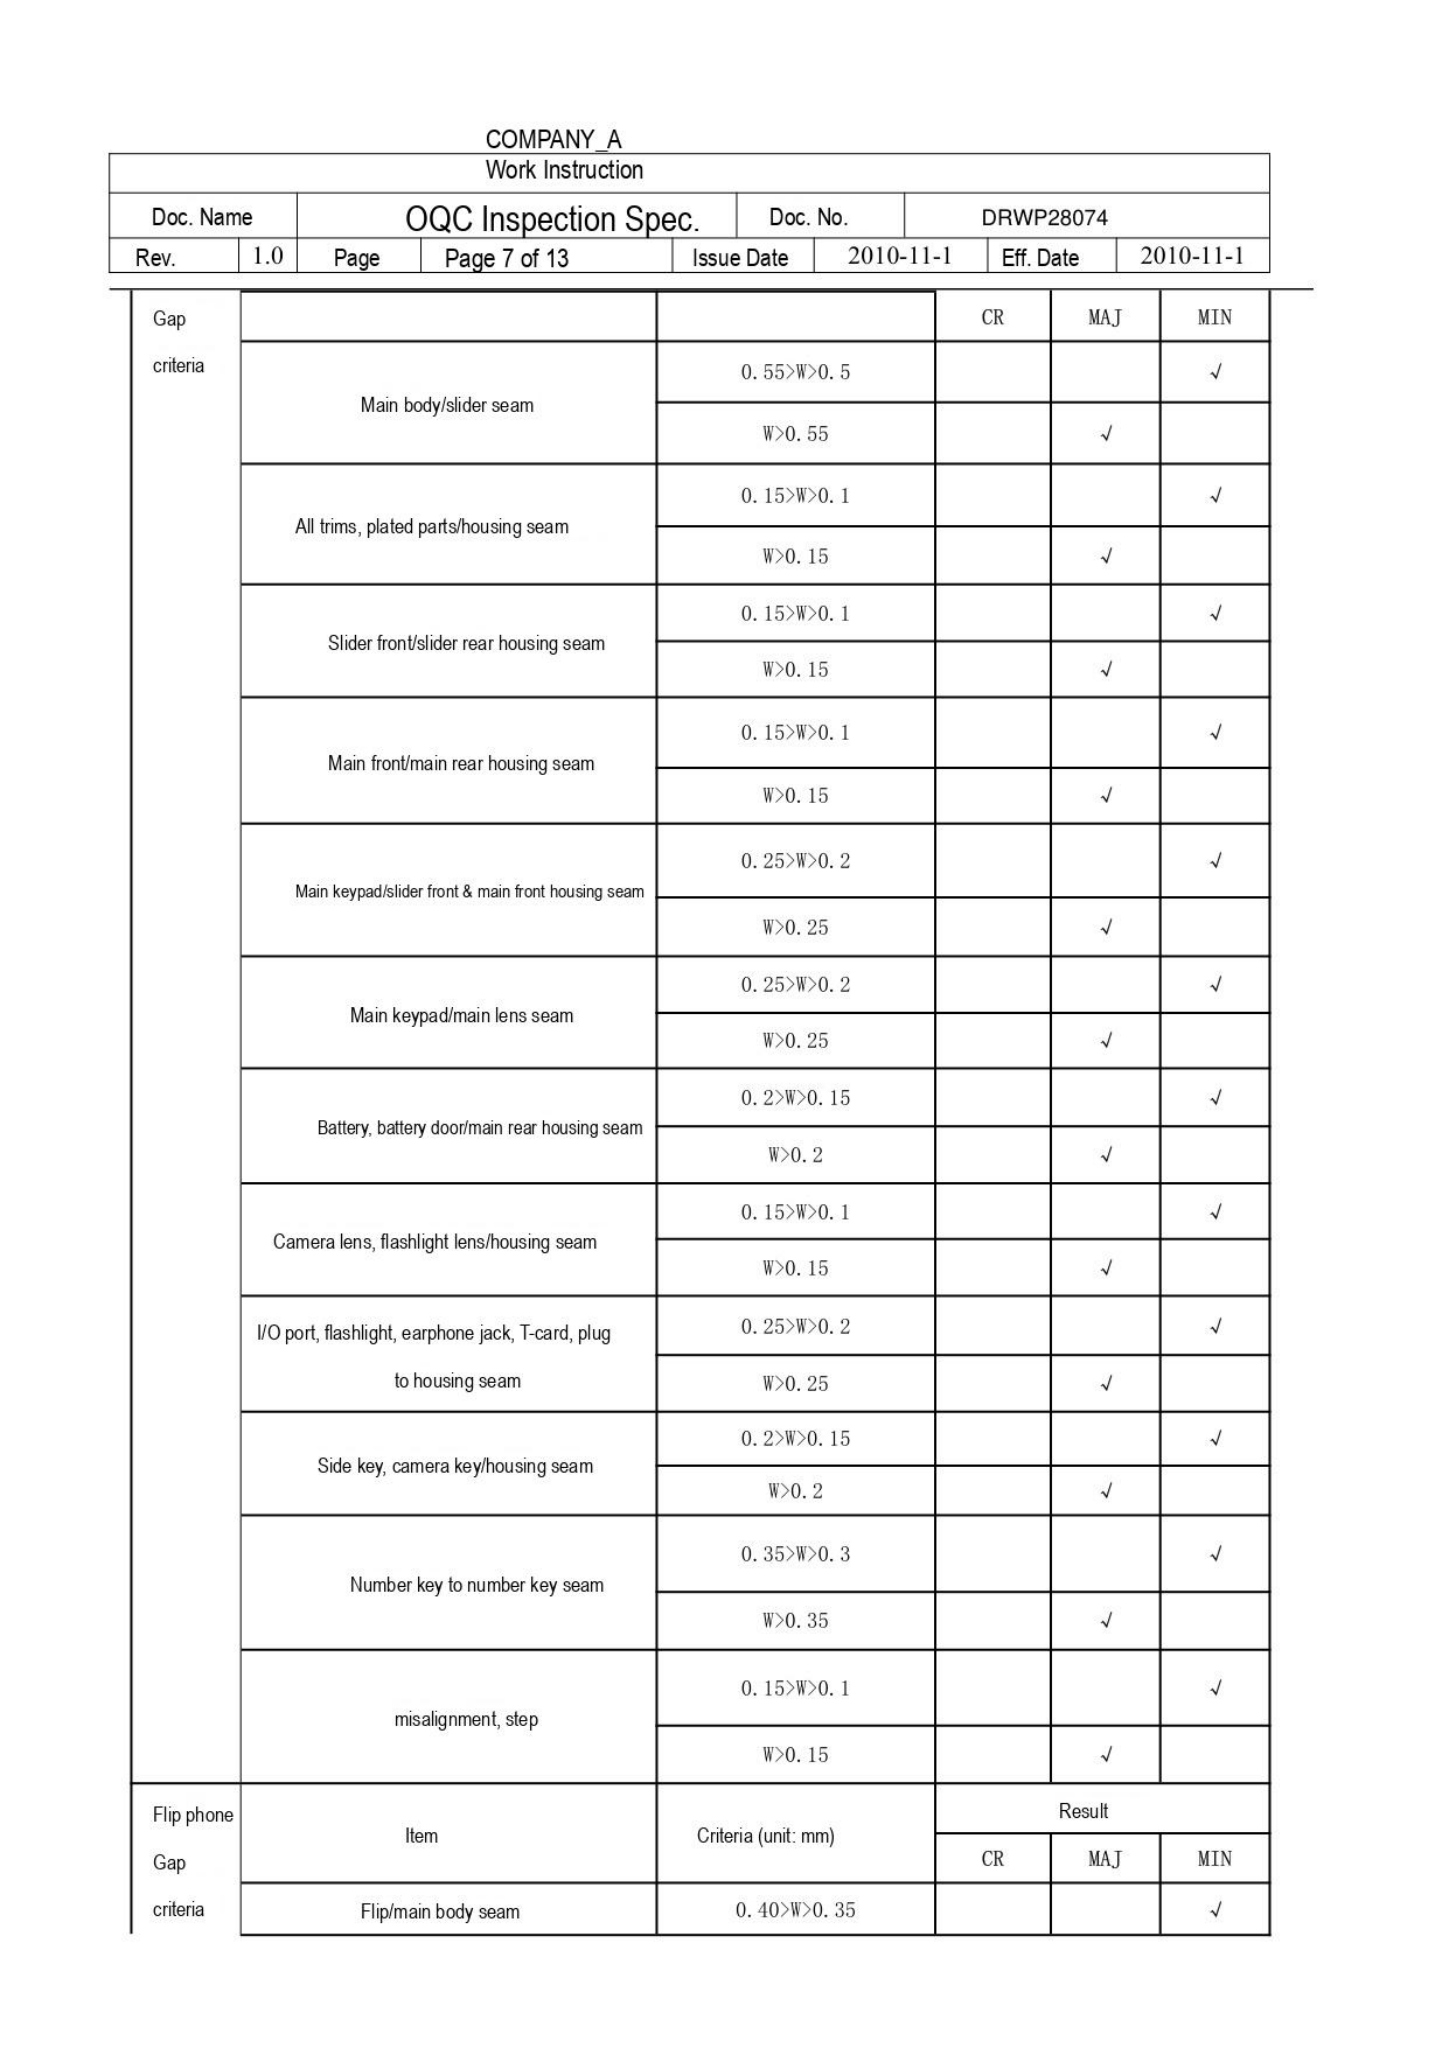COMPANY_A

| Work Instruction | | | | | | | |
|---|---|---|---|---|---|---|---|
| Doc. Name | OQC Inspection Spec. | | | Doc. No. | DRWP28074 | | |
| Rev. | 1.0 | Page | Page 7 of 13 | Issue Date | 2010-11-1 | Eff. Date | 2010-11-1 |

| Gap criteria | | | CR | MAJ | MIN |
|---|---|---|---|---|---|
| | Main body/slider seam | 0. 55>W>0. 5 | | | √ |
| | | W>0. 55 | | √ | |
| | All trims, plated parts/housing seam | 0. 15>W>0. 1 | | | √ |
| | | W>0. 15 | | √ | |
| | Slider front/slider rear housing seam | 0. 15>W>0. 1 | | | √ |
| | | W>0. 15 | | √ | |
| | Main front/main rear housing seam | 0. 15>W>0. 1 | | | √ |
| | | W>0. 15 | | √ | |
| | Main keypad/slider front & main front housing seam | 0. 25>W>0. 2 | | | √ |
| | | W>0. 25 | | √ | |
| | Main keypad/main lens seam | 0. 25>W>0. 2 | | | √ |
| | | W>0. 25 | | √ | |
| | Battery, battery door/main rear housing seam | 0. 2>W>0. 15 | | | √ |
| | | W>0. 2 | | √ | |
| | Camera lens, flashlight lens/housing seam | 0. 15>W>0. 1 | | | √ |
| | | W>0. 15 | | √ | |
| | I/O port, flashlight, earphone jack, T-card, plug to housing seam | 0. 25>W>0. 2 | | | √ |
| | | W>0. 25 | | √ | |
| | Side key, camera key/housing seam | 0. 2>W>0. 15 | | | √ |
| | | W>0. 2 | | √ | |
| | Number key to number key seam | 0. 35>W>0. 3 | | | √ |
| | | W>0. 35 | | √ | |
| | misalignment, step | 0. 15>W>0. 1 | | | √ |
| | | W>0. 15 | | √ | |

| Flip phone Gap criteria | Item | Criteria (unit: mm) | Result | | |
|---|---|---|---|---|---|
| | | | CR | MAJ | MIN |
| | Flip/main body seam | 0. 40>W>0. 35 | | | √ |
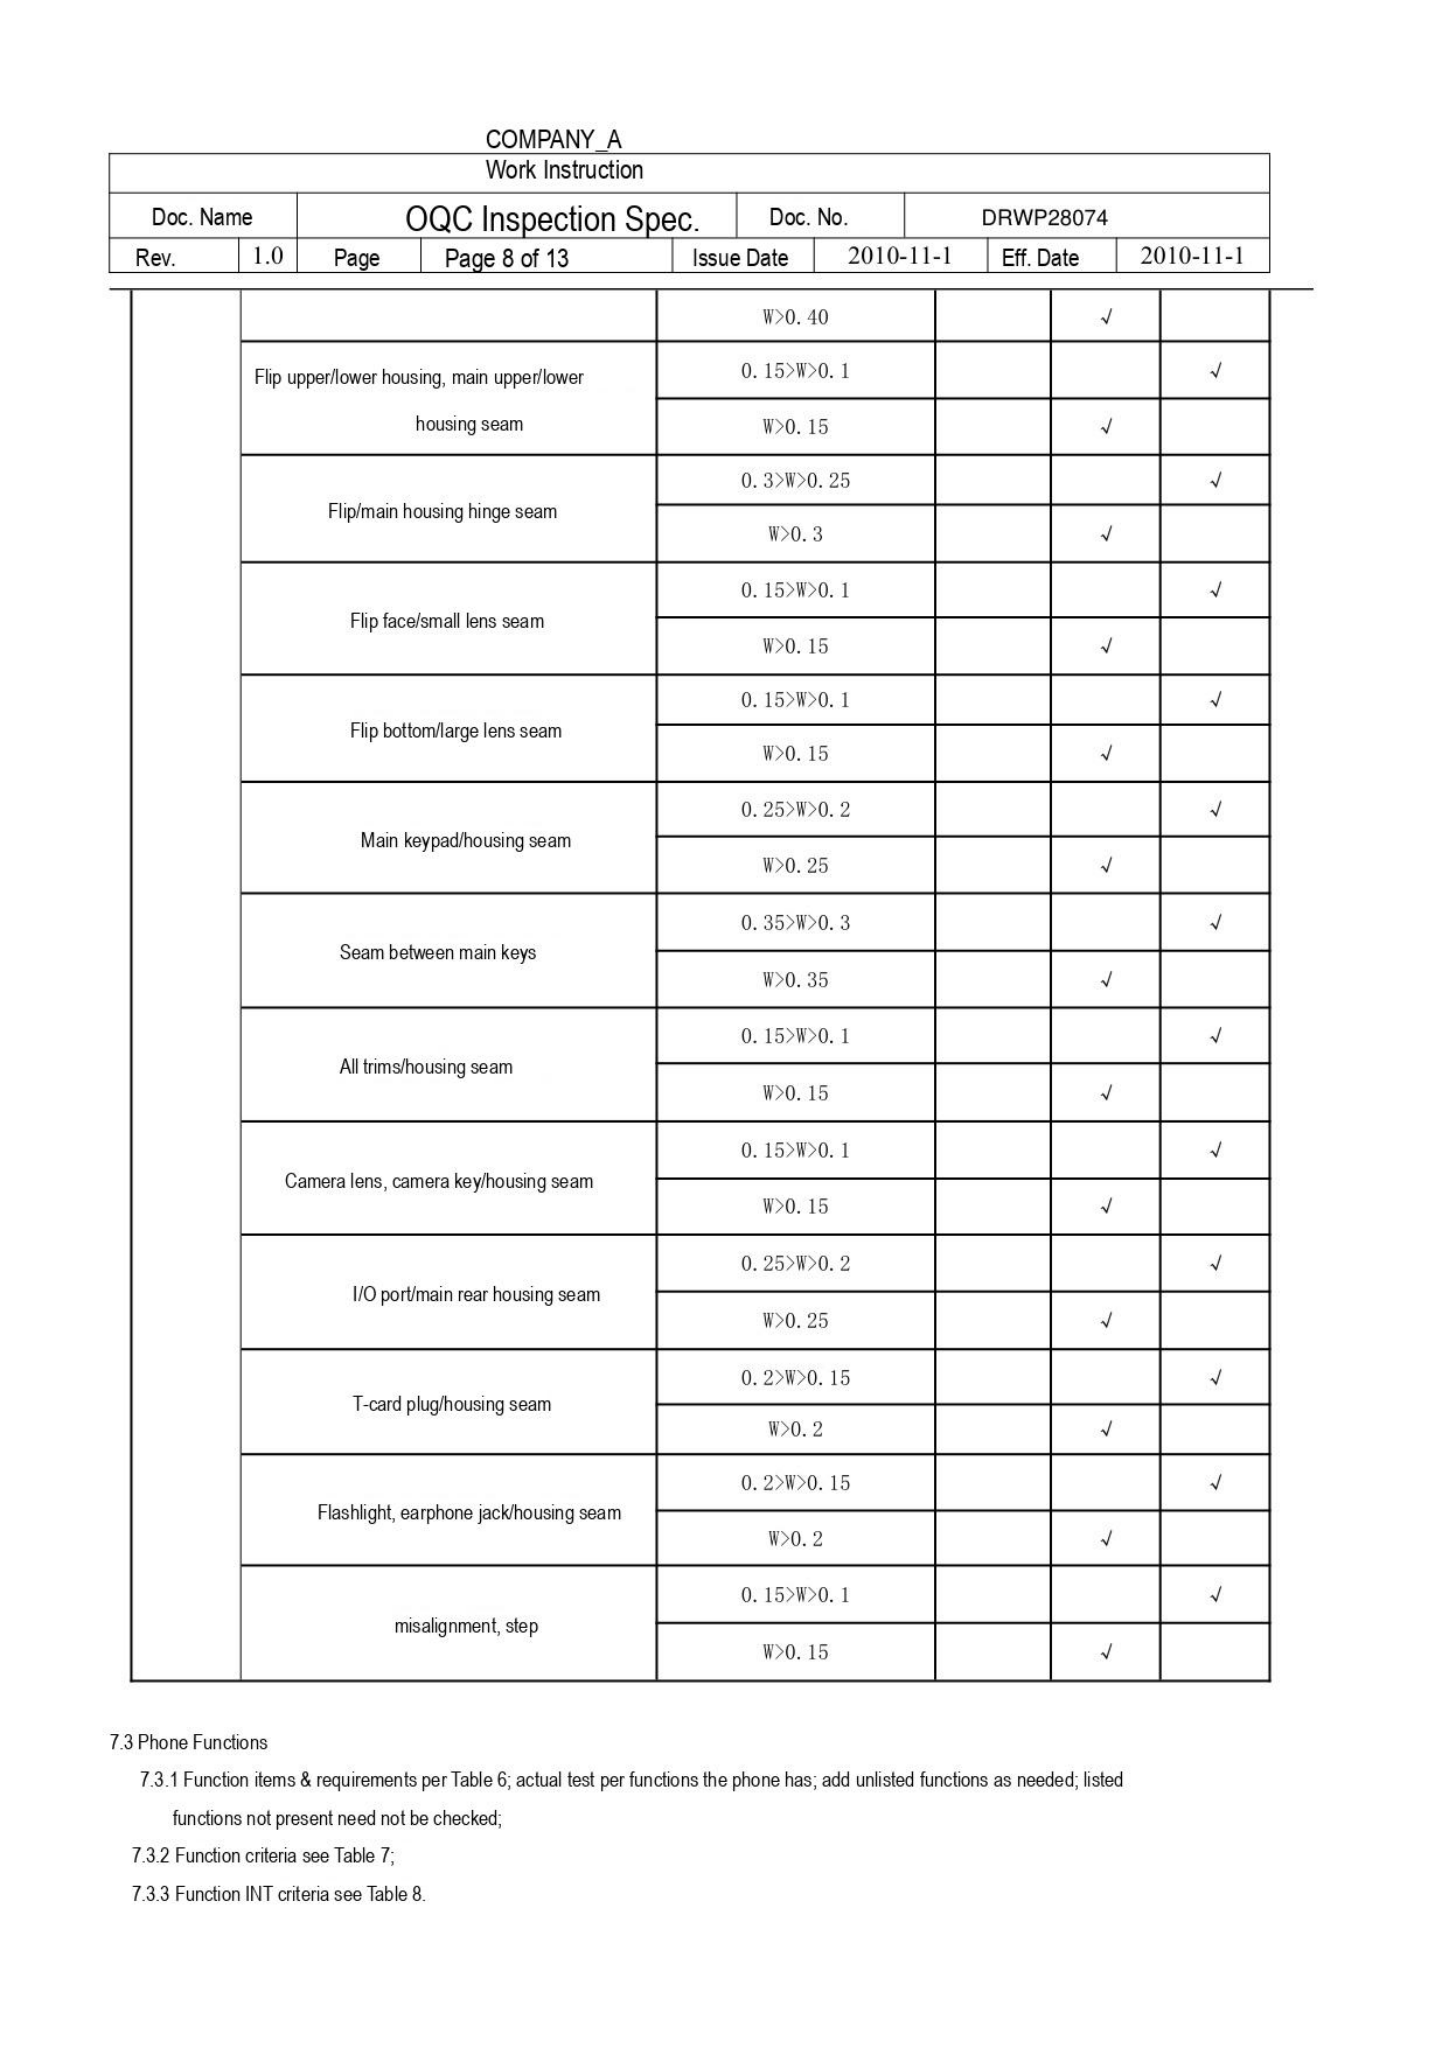COMPANY_A

| Work Instruction | | | | | | | |
|---|---|---|---|---|---|---|---|
| Doc. Name | | OQC Inspection Spec. | | Doc. No. | | DRWP28074 | |
| Rev. | 1.0 | Page | Page 8 of 13 | Issue Date | 2010-11-1 | Eff. Date | 2010-11-1 |

| | | | | | |
|---|---|---|---|---|---|
| | | W>0.40 | | √ | |
| | Flip upper/lower housing, main upper/lower housing seam | 0.15>W>0.1 | | | √ |
| | | W>0.15 | | √ | |
| | Flip/main housing hinge seam | 0.3>W>0.25 | | | √ |
| | | W>0.3 | | √ | |
| | Flip face/small lens seam | 0.15>W>0.1 | | | √ |
| | | W>0.15 | | √ | |
| | Flip bottom/large lens seam | 0.15>W>0.1 | | | √ |
| | | W>0.15 | | √ | |
| | Main keypad/housing seam | 0.25>W>0.2 | | | √ |
| | | W>0.25 | | √ | |
| | Seam between main keys | 0.35>W>0.3 | | | √ |
| | | W>0.35 | | √ | |
| | All trims/housing seam | 0.15>W>0.1 | | | √ |
| | | W>0.15 | | √ | |
| | Camera lens, camera key/housing seam | 0.15>W>0.1 | | | √ |
| | | W>0.15 | | √ | |
| | I/O port/main rear housing seam | 0.25>W>0.2 | | | √ |
| | | W>0.25 | | √ | |
| | T-card plug/housing seam | 0.2>W>0.15 | | | √ |
| | | W>0.2 | | √ | |
| | Flashlight, earphone jack/housing seam | 0.2>W>0.15 | | | √ |
| | | W>0.2 | | √ | |
| | misalignment, step | 0.15>W>0.1 | | | √ |
| | | W>0.15 | | √ | |

7.3 Phone Functions

7.3.1 Function items & requirements per Table 6; actual test per functions the phone has; add unlisted functions as needed; listed functions not present need not be checked;

7.3.2 Function criteria see Table 7;

7.3.3 Function INT criteria see Table 8.
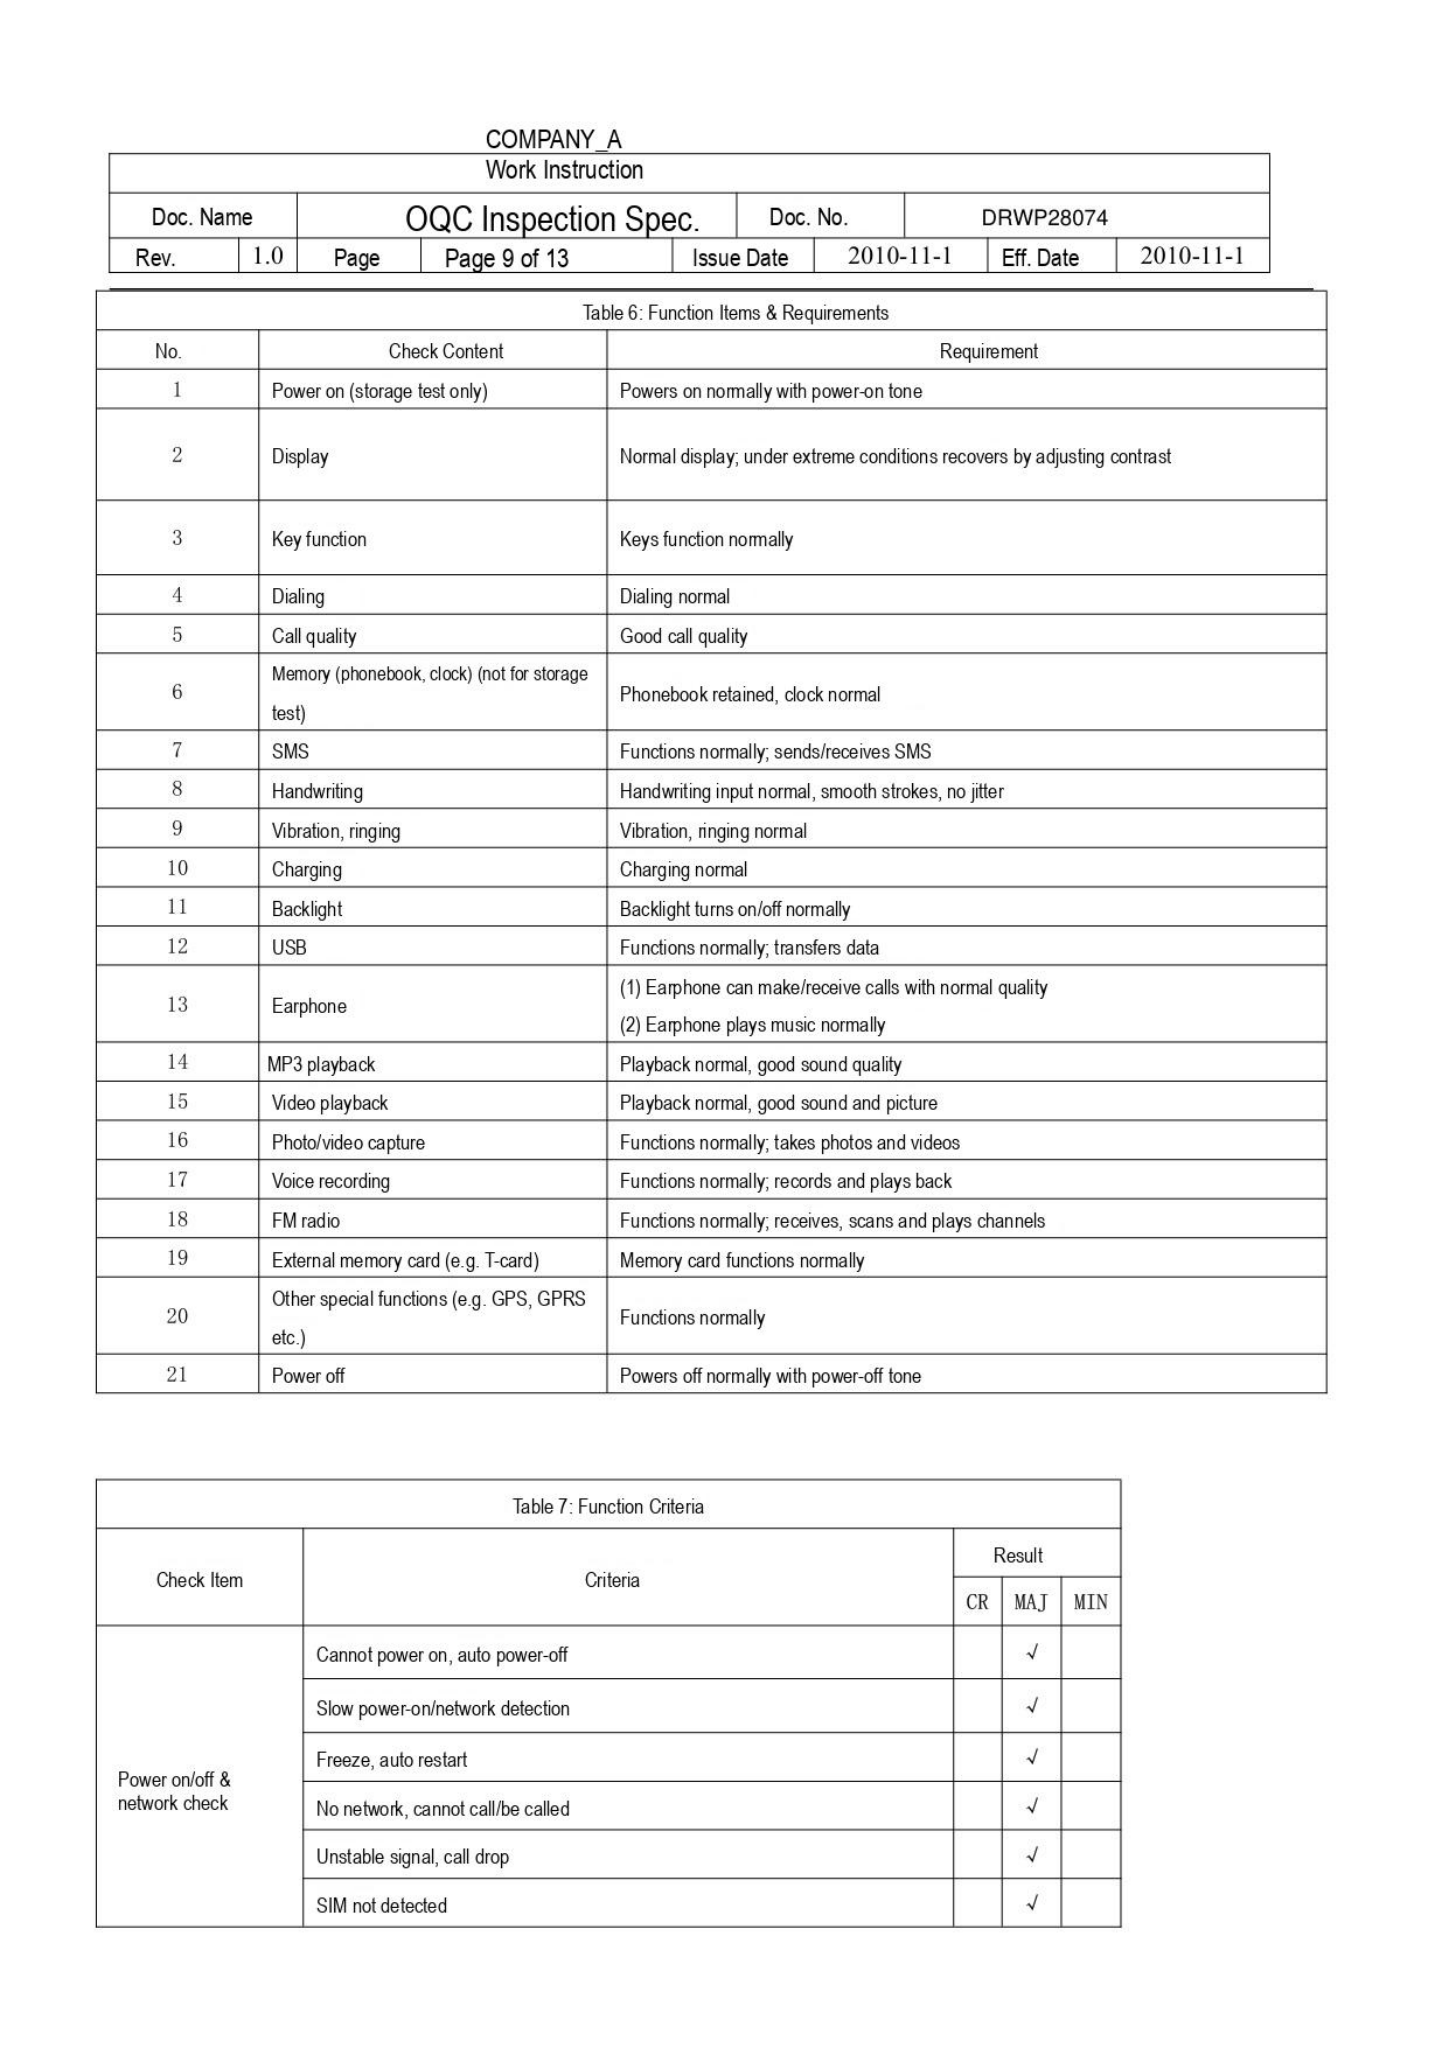COMPANY_A

| Work Instruction | | | | | | | |
|---|---|---|---|---|---|---|---|
| Doc. Name | | OQC Inspection Spec. | | Doc. No. | | DRWP28074 | |
| Rev. | 1.0 | Page | Page 9 of 13 | Issue Date | 2010-11-1 | Eff. Date | 2010-11-1 |

Table 6: Function Items & Requirements

| No. | Check Content | Requirement |
|---|---|---|
| 1 | Power on (storage test only) | Powers on normally with power-on tone |
| 2 | Display | Normal display; under extreme conditions recovers by adjusting contrast |
| 3 | Key function | Keys function normally |
| 4 | Dialing | Dialing normal |
| 5 | Call quality | Good call quality |
| 6 | Memory (phonebook, clock) (not for storage test) | Phonebook retained, clock normal |
| 7 | SMS | Functions normally; sends/receives SMS |
| 8 | Handwriting | Handwriting input normal, smooth strokes, no jitter |
| 9 | Vibration, ringing | Vibration, ringing normal |
| 10 | Charging | Charging normal |
| 11 | Backlight | Backlight turns on/off normally |
| 12 | USB | Functions normally; transfers data |
| 13 | Earphone | (1) Earphone can make/receive calls with normal quality<br>(2) Earphone plays music normally |
| 14 | MP3 playback | Playback normal, good sound quality |
| 15 | Video playback | Playback normal, good sound and picture |
| 16 | Photo/video capture | Functions normally; takes photos and videos |
| 17 | Voice recording | Functions normally; records and plays back |
| 18 | FM radio | Functions normally; receives, scans and plays channels |
| 19 | External memory card (e.g. T-card) | Memory card functions normally |
| 20 | Other special functions (e.g. GPS, GPRS etc.) | Functions normally |
| 21 | Power off | Powers off normally with power-off tone |

Table 7: Function Criteria

| Check Item | Criteria | Result: CR | Result: MAJ | Result: MIN |
|---|---|---|---|---|
| Power on/off & network check | Cannot power on, auto power-off | | √ | |
| | Slow power-on/network detection | | √ | |
| | Freeze, auto restart | | √ | |
| | No network, cannot call/be called | | √ | |
| | Unstable signal, call drop | | √ | |
| | SIM not detected | | √ | |
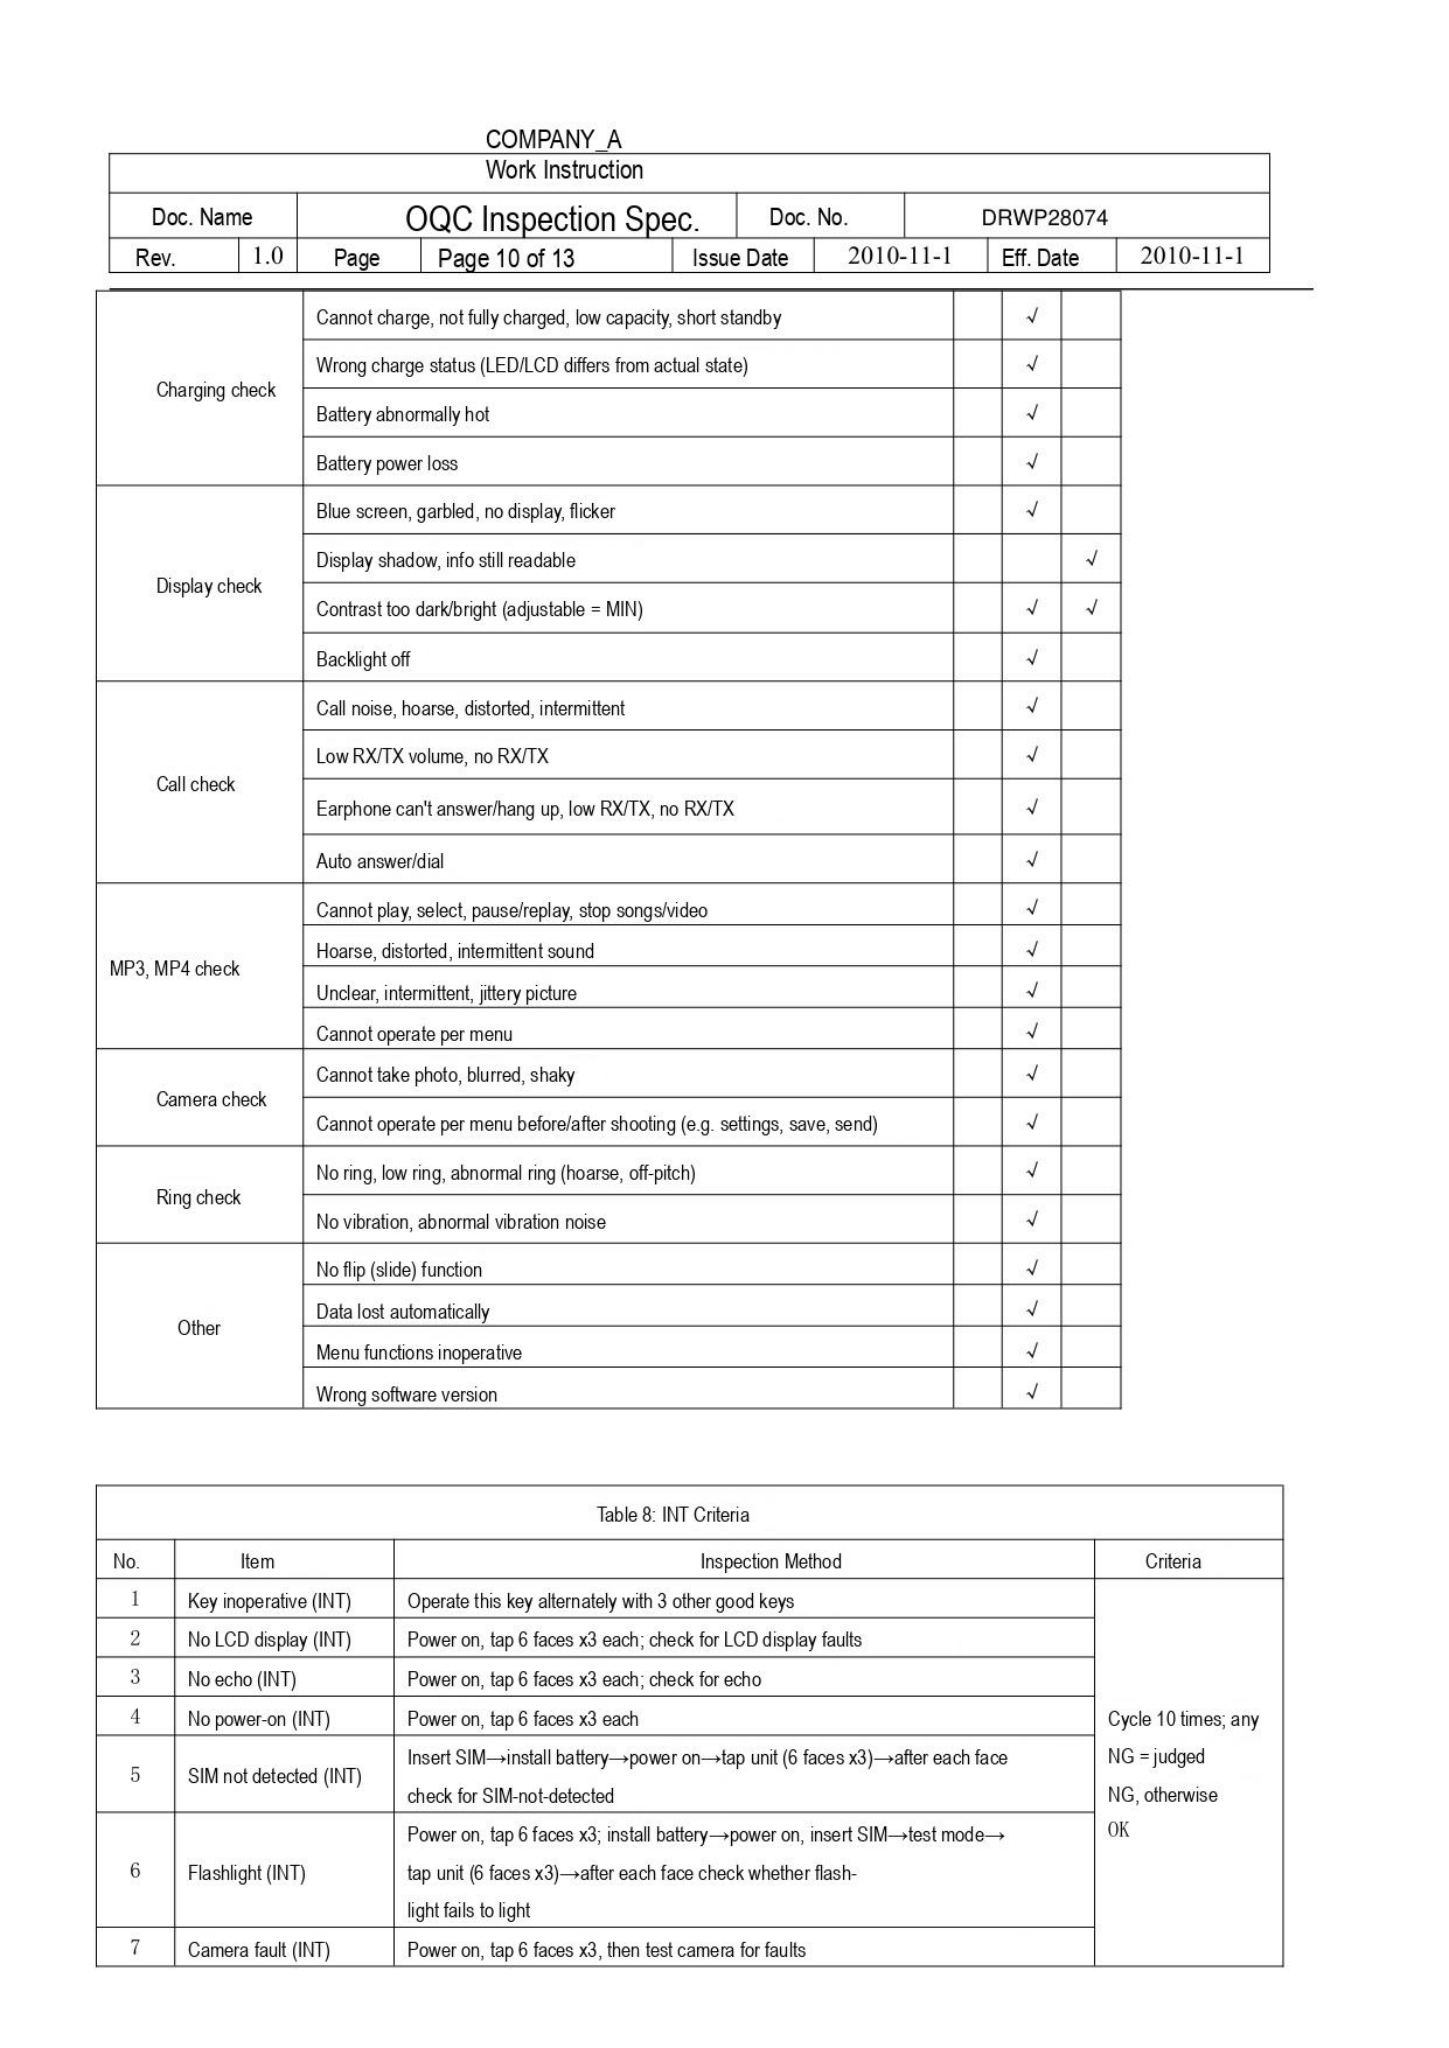COMPANY_A

| Work Instruction | | | | | | | |
|---|---|---|---|---|---|---|---|
| Doc. Name | | OQC Inspection Spec. | | Doc. No. | DRWP28074 | | |
| Rev. | 1.0 | Page | Page 10 of 13 | Issue Date | 2010-11-1 | Eff. Date | 2010-11-1 |

| | | | | |
|---|---|---|---|---|
| Charging check | Cannot charge, not fully charged, low capacity, short standby | | √ | |
| | Wrong charge status (LED/LCD differs from actual state) | | √ | |
| | Battery abnormally hot | | √ | |
| | Battery power loss | | √ | |
| Display check | Blue screen, garbled, no display, flicker | | √ | |
| | Display shadow, info still readable | | | √ |
| | Contrast too dark/bright (adjustable = MIN) | | √ | √ |
| | Backlight off | | √ | |
| Call check | Call noise, hoarse, distorted, intermittent | | √ | |
| | Low RX/TX volume, no RX/TX | | √ | |
| | Earphone can't answer/hang up, low RX/TX, no RX/TX | | √ | |
| | Auto answer/dial | | √ | |
| MP3, MP4 check | Cannot play, select, pause/replay, stop songs/video | | √ | |
| | Hoarse, distorted, intermittent sound | | √ | |
| | Unclear, intermittent, jittery picture | | √ | |
| | Cannot operate per menu | | √ | |
| Camera check | Cannot take photo, blurred, shaky | | √ | |
| | Cannot operate per menu before/after shooting (e.g. settings, save, send) | | √ | |
| Ring check | No ring, low ring, abnormal ring (hoarse, off-pitch) | | √ | |
| | No vibration, abnormal vibration noise | | √ | |
| Other | No flip (slide) function | | √ | |
| | Data lost automatically | | √ | |
| | Menu functions inoperative | | √ | |
| | Wrong software version | | √ | |

| Table 8: INT Criteria | | | |
|---|---|---|---|
| No. | Item | Inspection Method | Criteria |
| 1 | Key inoperative (INT) | Operate this key alternately with 3 other good keys | Cycle 10 times; any NG = judged NG, otherwise OK |
| 2 | No LCD display (INT) | Power on, tap 6 faces x3 each; check for LCD display faults | |
| 3 | No echo (INT) | Power on, tap 6 faces x3 each; check for echo | |
| 4 | No power-on (INT) | Power on, tap 6 faces x3 each | |
| 5 | SIM not detected (INT) | Insert SIM→install battery→power on→tap unit (6 faces x3)→after each face check for SIM-not-detected | |
| 6 | Flashlight (INT) | Power on, tap 6 faces x3; install battery→power on, insert SIM→test mode→tap unit (6 faces x3)→after each face check whether flash-light fails to light | |
| 7 | Camera fault (INT) | Power on, tap 6 faces x3, then test camera for faults | |
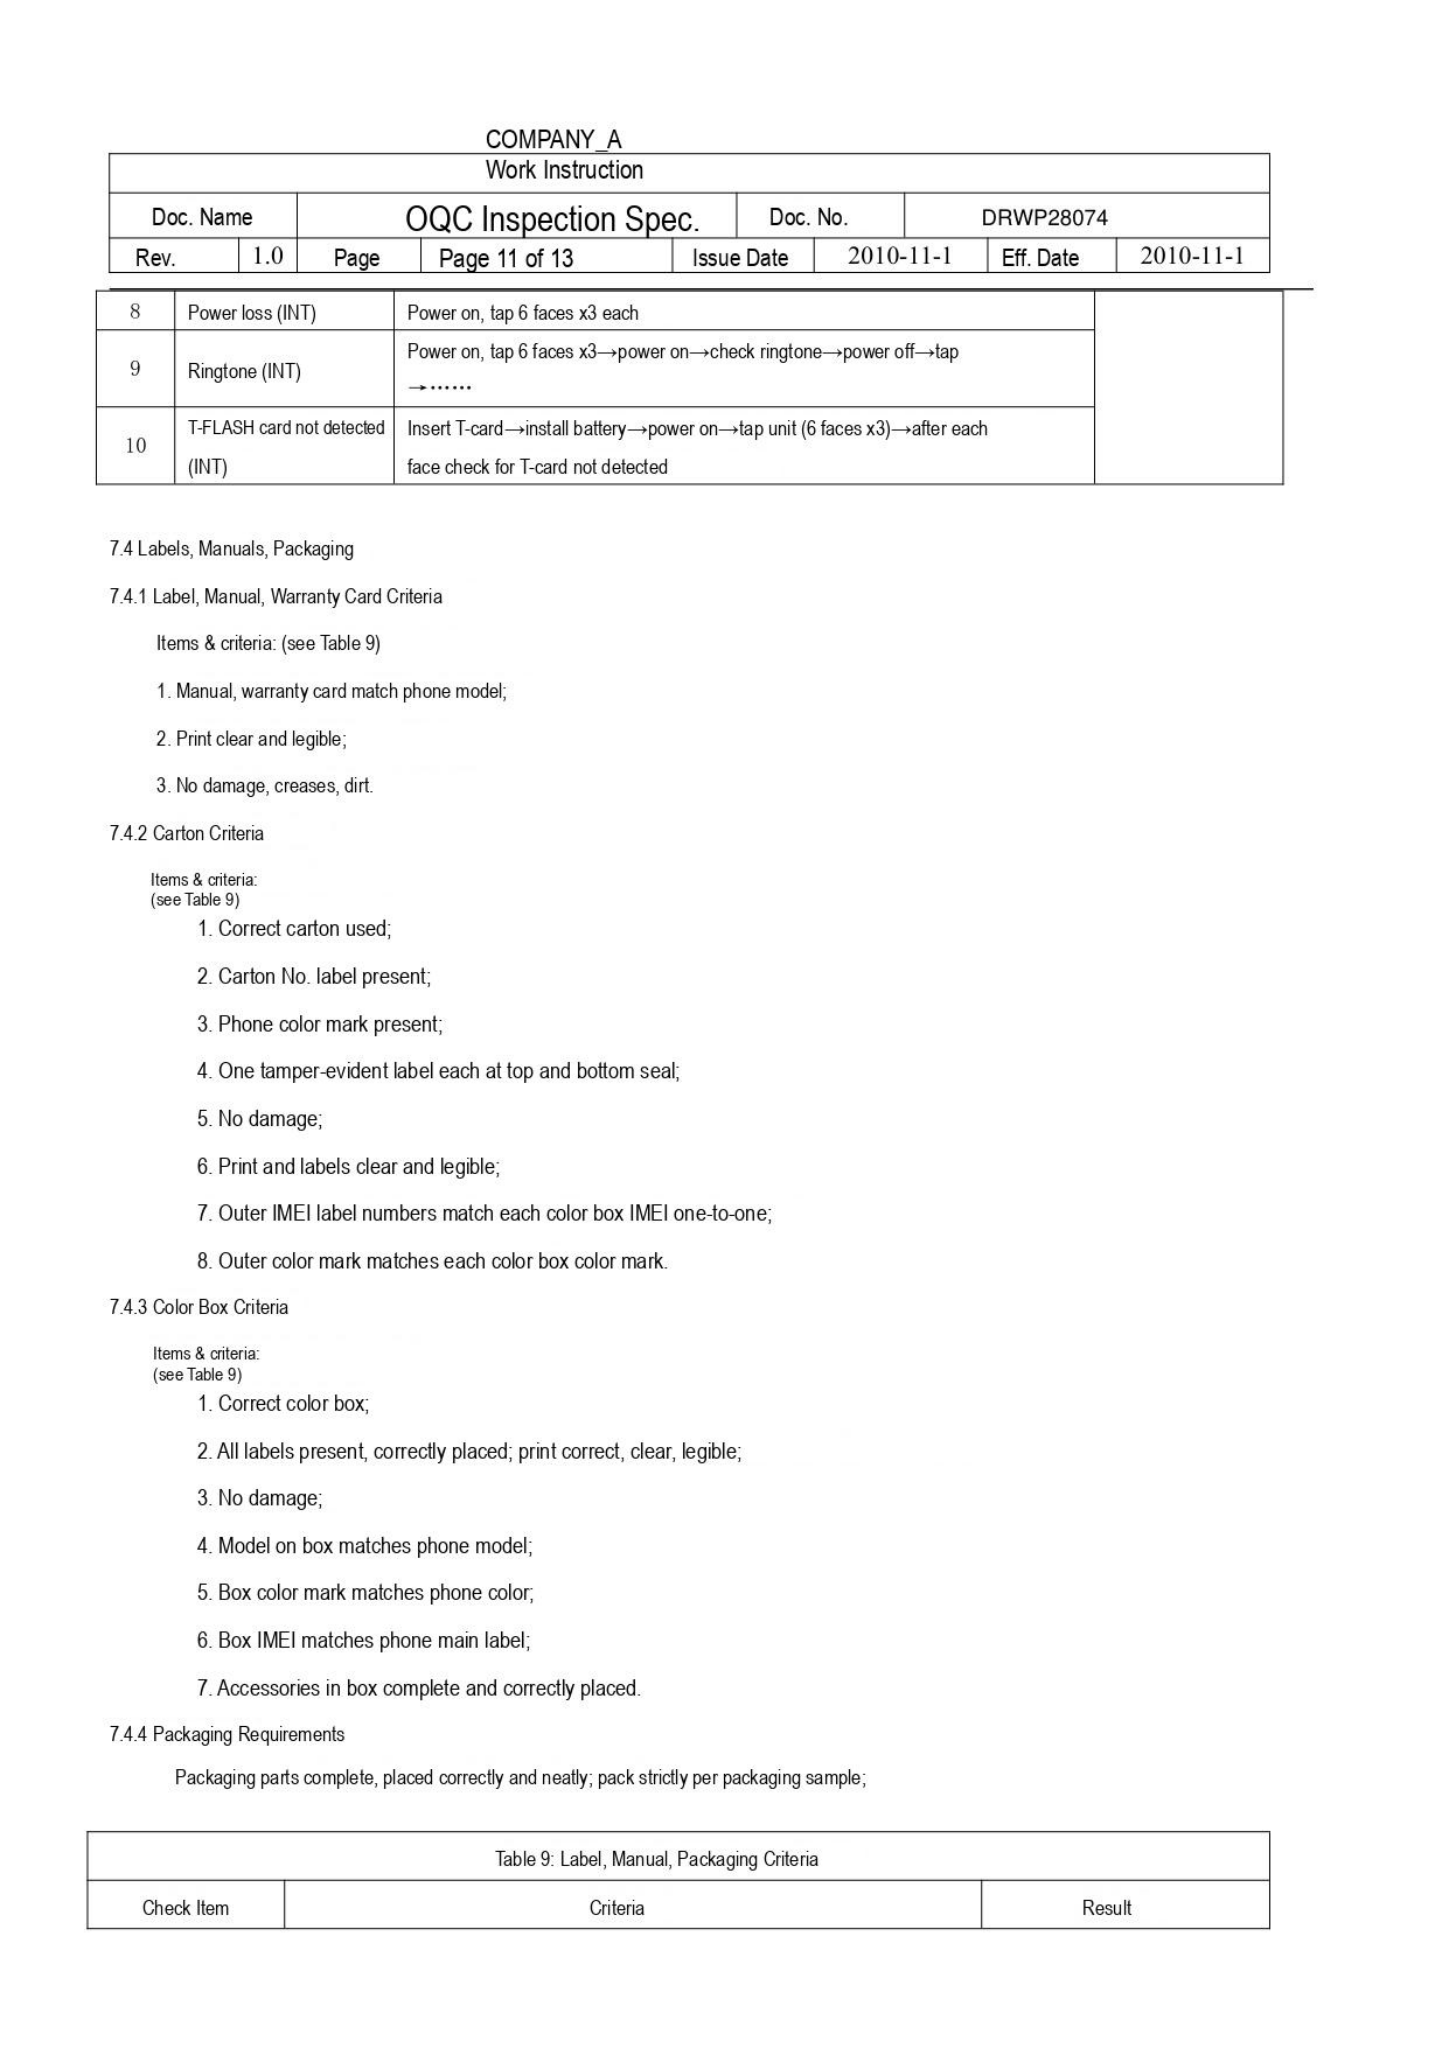COMPANY_A

| Work Instruction | | | | | | | |
|---|---|---|---|---|---|---|---|
| Doc. Name | | OQC Inspection Spec. | | Doc. No. | DRWP28074 | | |
| Rev. | 1.0 | Page | Page 11 of 13 | Issue Date | 2010-11-1 | Eff. Date | 2010-11-1 |

| | | | |
|---|---|---|---|
| 8 | Power loss (INT) | Power on, tap 6 faces x3 each | |
| 9 | Ringtone (INT) | Power on, tap 6 faces x3→power on→check ringtone→power off→tap →…… | |
| 10 | T-FLASH card not detected (INT) | Insert T-card→install battery→power on→tap unit (6 faces x3)→after each face check for T-card not detected | |

7.4 Labels, Manuals, Packaging

7.4.1 Label, Manual, Warranty Card Criteria

Items & criteria: (see Table 9)

1. Manual, warranty card match phone model;

2. Print clear and legible;

3. No damage, creases, dirt.

7.4.2 Carton Criteria

Items & criteria:
(see Table 9)

1. Correct carton used;

2. Carton No. label present;

3. Phone color mark present;

4. One tamper-evident label each at top and bottom seal;

5. No damage;

6. Print and labels clear and legible;

7. Outer IMEI label numbers match each color box IMEI one-to-one;

8. Outer color mark matches each color box color mark.

7.4.3 Color Box Criteria

Items & criteria:
(see Table 9)

1. Correct color box;

2. All labels present, correctly placed; print correct, clear, legible;

3. No damage;

4. Model on box matches phone model;

5. Box color mark matches phone color;

6. Box IMEI matches phone main label;

7. Accessories in box complete and correctly placed.

7.4.4 Packaging Requirements

Packaging parts complete, placed correctly and neatly; pack strictly per packaging sample;

| Table 9: Label, Manual, Packaging Criteria | | |
|---|---|---|
| Check Item | Criteria | Result |
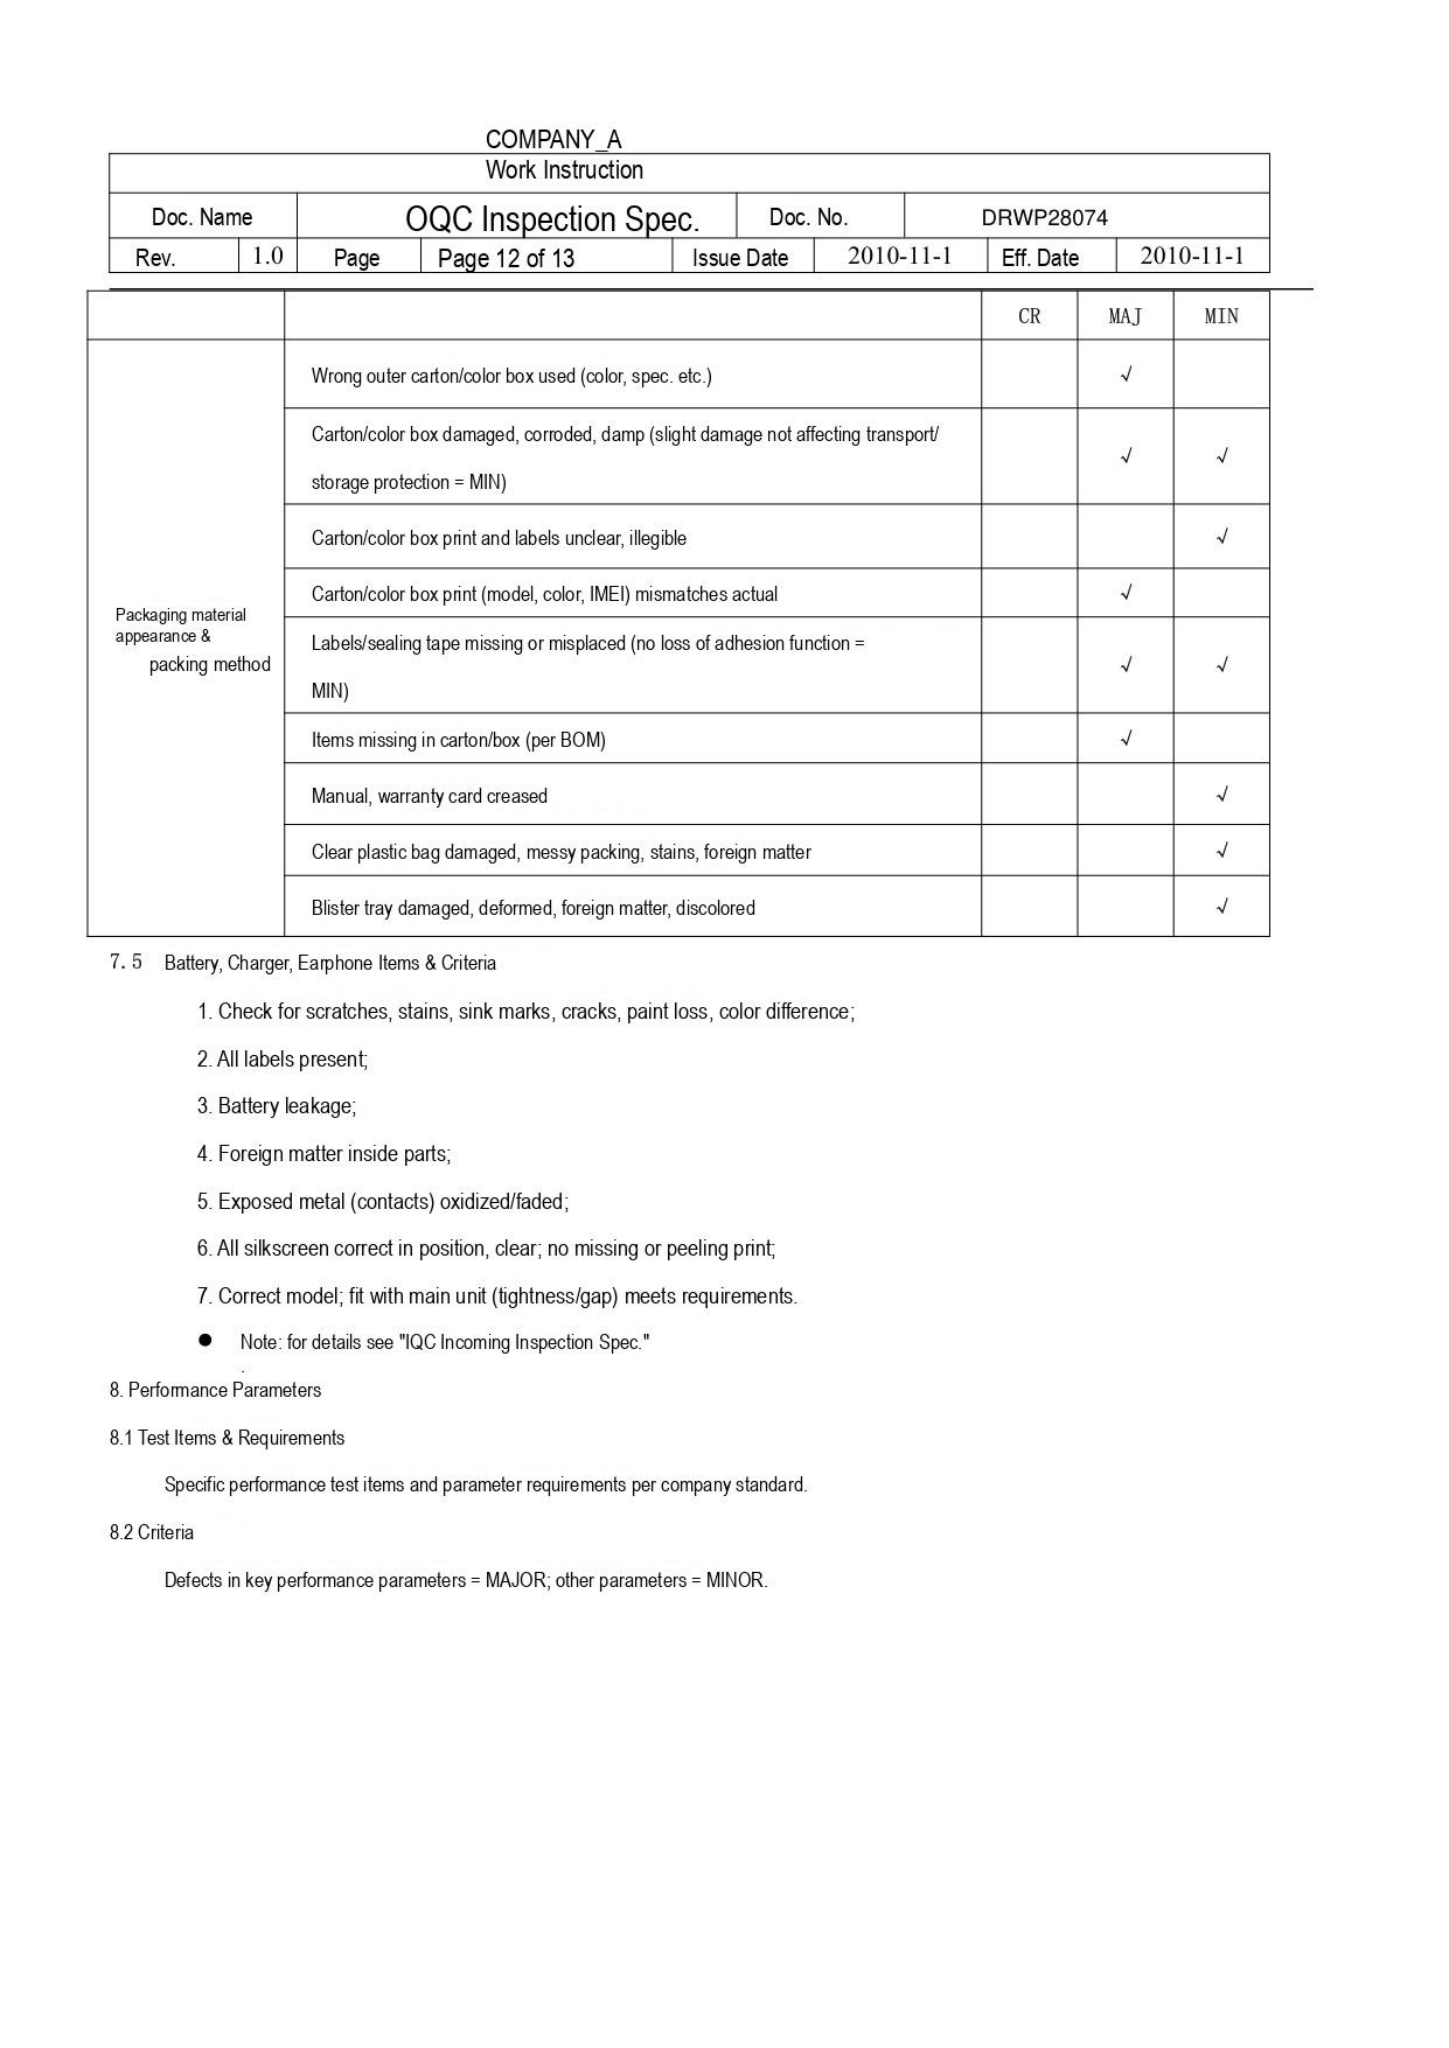COMPANY_A

| Work Instruction | | | | | | | |
|---|---|---|---|---|---|---|---|
| Doc. Name | | OQC Inspection Spec. | | Doc. No. | | DRWP28074 | |
| Rev. | 1.0 | Page | Page 12 of 13 | Issue Date | 2010-11-1 | Eff. Date | 2010-11-1 |

| | | CR | MAJ | MIN |
|---|---|---|---|---|
| Packaging material appearance & packing method | Wrong outer carton/color box used (color, spec. etc.) | | √ | |
| | Carton/color box damaged, corroded, damp (slight damage not affecting transport/ storage protection = MIN) | | √ | √ |
| | Carton/color box print and labels unclear, illegible | | | √ |
| | Carton/color box print (model, color, IMEI) mismatches actual | | √ | |
| | Labels/sealing tape missing or misplaced (no loss of adhesion function = MIN) | | √ | √ |
| | Items missing in carton/box (per BOM) | | √ | |
| | Manual, warranty card creased | | | √ |
| | Clear plastic bag damaged, messy packing, stains, foreign matter | | | √ |
| | Blister tray damaged, deformed, foreign matter, discolored | | | √ |

7.5 Battery, Charger, Earphone Items & Criteria

1. Check for scratches, stains, sink marks, cracks, paint loss, color difference;
2. All labels present;
3. Battery leakage;
4. Foreign matter inside parts;
5. Exposed metal (contacts) oxidized/faded;
6. All silkscreen correct in position, clear; no missing or peeling print;
7. Correct model; fit with main unit (tightness/gap) meets requirements.

- Note: for details see "IQC Incoming Inspection Spec."

8. Performance Parameters

8.1 Test Items & Requirements

Specific performance test items and parameter requirements per company standard.

8.2 Criteria

Defects in key performance parameters = MAJOR; other parameters = MINOR.